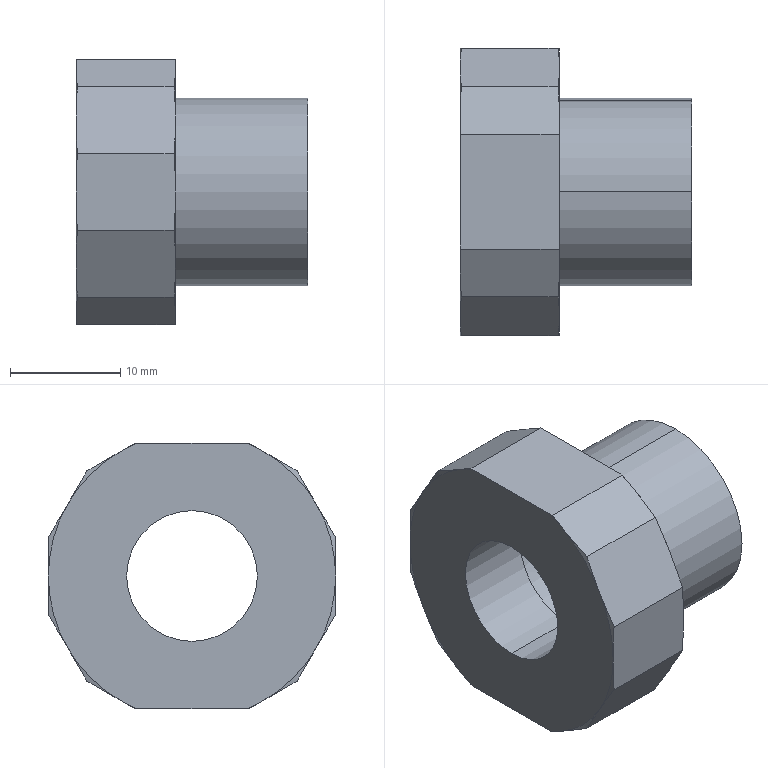Part | STEP file | 1_6 | 1 solid | 49 faces | box 21 x 26 x 24 mm | volume 4121 mm3 | cone 26 | plane 18 | cylinder 5 | commonest cylinder face diameters 17 x3 11.835 x2